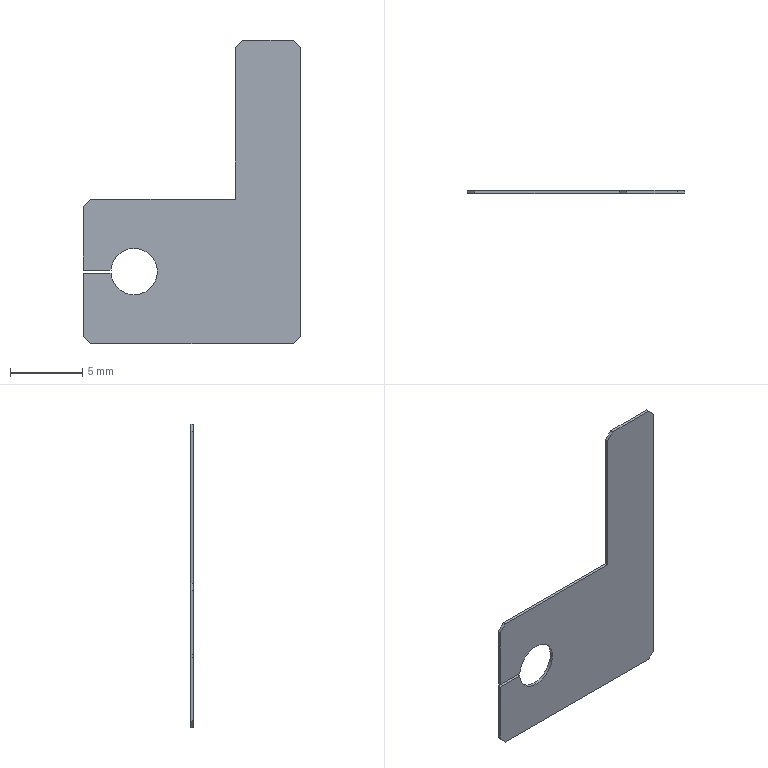Part | SolidWorks | features ICE 3, Chamfer 1, FlatPattern 1, SMBaseFlange 1, SheetMetal 1 | 1 solid | 19 faces | box 15 x 0.2 x 21 mm | volume 38.09 mm3 | plane 16 | cylinder 3 | commonest cylinder face diameters 3.2 x3
STEP:
#1=CARTESIAN_POINT('',(-5.597,0.,5.1));
#2=VERTEX_POINT('',#1);
#3=CARTESIAN_POINT('',(-4.,0.,6.6));
#4=VERTEX_POINT('',#3);
#5=CARTESIAN_POINT('',(-4.,0.,5.));
#6=DIRECTION('',(0.,1.,0.));
#7=DIRECTION('',(0.,0.,1.));
#8=AXIS2_PLACEMENT_3D('',#5,#6,#7);
#9=CIRCLE('',#8,1.6);
#10=EDGE_CURVE('',#2,#4,#9,.T.);
#11=ORIENTED_EDGE('',*,*,#10,.T.);
#12=CARTESIAN_POINT('',(-4.,-0.2,6.6));
#13=VERTEX_POINT('',#12);
#14=CARTESIAN_POINT('',(-4.,9.8,6.6));
#15=DIRECTION('',(0.,-1.,0.));
#16=VECTOR('',#15,1000.);
#17=LINE('',#14,#16);
#18=EDGE_CURVE('',#4,#13,#17,.T.);
#19=ORIENTED_EDGE('',*,*,#18,.T.);
#20=CARTESIAN_POINT('',(-5.597,-0.2,5.1));
#21=VERTEX_POINT('',#20);
#22=CARTESIAN_POINT('',(-4.,-0.2,5.));
#23=DIRECTION('',(0.,-1.,0.));
#24=DIRECTION('',(0.,0.,-1.));
#25=AXIS2_PLACEMENT_3D('',#22,#23,#24);
#26=CIRCLE('',#25,1.6);
#27=EDGE_CURVE('',#13,#21,#26,.T.);
#28=ORIENTED_EDGE('',*,*,#27,.T.);
#29=CARTESIAN_POINT('',(-5.597,0.,5.1));
#30=DIRECTION('',(0.,-1.,0.));
#31=VECTOR('',#30,1000.);
#32=LINE('',#29,#31);
#33=EDGE_CURVE('',#2,#21,#32,.T.);
#34=ORIENTED_EDGE('',*,*,#33,.F.);
#35=EDGE_LOOP('',(#11,#19,#28,#34));
#36=FACE_OUTER_BOUND('',#35,.T.);
#37=CARTESIAN_POINT('',(-4.,9.8,5.));
#38=DIRECTION('',(0.,-1.,0.));
#39=DIRECTION('',(0.,0.,-1.));
#40=AXIS2_PLACEMENT_3D('',#37,#38,#39);
#41=CYLINDRICAL_SURFACE('',#40,1.6);
#42=ADVANCED_FACE('',(#36),#41,.F.);
#43=ORIENTED_EDGE('',*,*,#18,.F.);
#44=CARTESIAN_POINT('',(-4.,0.,3.4));
#45=VERTEX_POINT('',#44);
#46=CARTESIAN_POINT('',(-4.,0.,5.));
#47=DIRECTION('',(0.,1.,0.));
#48=DIRECTION('',(0.,0.,1.));
#49=AXIS2_PLACEMENT_3D('',#46,#47,#48);
#50=CIRCLE('',#49,1.6);
#51=EDGE_CURVE('',#4,#45,#50,.T.);
#52=ORIENTED_EDGE('',*,*,#51,.T.);
#53=CARTESIAN_POINT('',(-4.,-0.2,3.4));
#54=VERTEX_POINT('',#53);
#55=CARTESIAN_POINT('',(-4.,9.8,3.4));
#56=DIRECTION('',(0.,-1.,0.));
#57=VECTOR('',#56,1000.);
#58=LINE('',#55,#57);
#59=EDGE_CURVE('',#45,#54,#58,.T.);
#60=ORIENTED_EDGE('',*,*,#59,.T.);
#61=CARTESIAN_POINT('',(-4.,-0.2,5.));
#62=DIRECTION('',(0.,-1.,0.));
#63=DIRECTION('',(0.,0.,-1.));
#64=AXIS2_PLACEMENT_3D('',#61,#62,#63);
#65=CIRCLE('',#64,1.6);
#66=EDGE_CURVE('',#54,#13,#65,.T.);
#67=ORIENTED_EDGE('',*,*,#66,.T.);
#68=EDGE_LOOP('',(#43,#52,#60,#67));
#69=FACE_OUTER_BOUND('',#68,.T.);
#70=CARTESIAN_POINT('',(-4.,9.8,5.));
#71=DIRECTION('',(0.,-1.,0.));
#72=DIRECTION('',(0.,0.,-1.));
#73=AXIS2_PLACEMENT_3D('',#70,#71,#72);
#74=CYLINDRICAL_SURFACE('',#73,1.6);
#75=ADVANCED_FACE('',(#69),#74,.F.);
#76=CARTESIAN_POINT('',(-7.,-0.2,10.));
#77=VERTEX_POINT('',#76);
#78=CARTESIAN_POINT('',(3.,-0.2,10.));
#79=VERTEX_POINT('',#78);
#80=CARTESIAN_POINT('',(-7.5,-0.2,10.));
#81=DIRECTION('',(1.,0.,0.));
#82=VECTOR('',#81,1000.);
#83=LINE('',#80,#82);
#84=EDGE_CURVE('',#77,#79,#83,.T.);
#85=ORIENTED_EDGE('',*,*,#84,.F.);
#86=CARTESIAN_POINT('',(-7.5,-0.2,9.5));
#87=VERTEX_POINT('',#86);
#88=CARTESIAN_POINT('',(-7.,-0.2,10.));
#89=DIRECTION('',(-0.7071,0.,-0.7071));
#90=VECTOR('',#89,1000.);
#91=LINE('',#88,#90);
#92=EDGE_CURVE('',#77,#87,#91,.T.);
#93=ORIENTED_EDGE('',*,*,#92,.T.);
#94=CARTESIAN_POINT('',(-7.5,-0.2,5.1));
#95=VERTEX_POINT('',#94);
#96=CARTESIAN_POINT('',(-7.5,-0.2,21.));
#97=DIRECTION('',(0.,0.,-1.));
#98=VECTOR('',#97,1000.);
#99=LINE('',#96,#98);
#100=EDGE_CURVE('',#87,#95,#99,.T.);
#101=ORIENTED_EDGE('',*,*,#100,.T.);
#102=CARTESIAN_POINT('',(-7.5,-0.2,5.1));
#103=DIRECTION('',(1.,0.,0.));
#104=VECTOR('',#103,1000.);
#105=LINE('',#102,#104);
#106=EDGE_CURVE('',#95,#21,#105,.T.);
#107=ORIENTED_EDGE('',*,*,#106,.T.);
#108=ORIENTED_EDGE('',*,*,#27,.F.);
#109=ORIENTED_EDGE('',*,*,#66,.F.);
#110=CARTESIAN_POINT('',(-5.597,-0.2,4.9));
#111=VERTEX_POINT('',#110);
#112=CARTESIAN_POINT('',(-4.,-0.2,5.));
#113=DIRECTION('',(0.,-1.,0.));
#114=DIRECTION('',(0.,0.,-1.));
#115=AXIS2_PLACEMENT_3D('',#112,#113,#114);
#116=CIRCLE('',#115,1.6);
#117=EDGE_CURVE('',#111,#54,#116,.T.);
#118=ORIENTED_EDGE('',*,*,#117,.F.);
#119=CARTESIAN_POINT('',(-7.5,-0.2,4.9));
#120=VERTEX_POINT('',#119);
#121=CARTESIAN_POINT('',(-7.5,-0.2,4.9));
#122=DIRECTION('',(-1.,0.,0.));
#123=VECTOR('',#122,1000.);
#124=LINE('',#121,#123);
#125=EDGE_CURVE('',#111,#120,#124,.T.);
#126=ORIENTED_EDGE('',*,*,#125,.T.);
#127=CARTESIAN_POINT('',(-7.5,-0.2,0.5));
#128=VERTEX_POINT('',#127);
#129=CARTESIAN_POINT('',(-7.5,-0.2,21.));
#130=DIRECTION('',(0.,0.,-1.));
#131=VECTOR('',#130,1000.);
#132=LINE('',#129,#131);
#133=EDGE_CURVE('',#120,#128,#132,.T.);
#134=ORIENTED_EDGE('',*,*,#133,.T.);
#135=CARTESIAN_POINT('',(-7.,-0.2,0.));
#136=VERTEX_POINT('',#135);
#137=CARTESIAN_POINT('',(-7.,-0.2,0.));
#138=DIRECTION('',(0.7071,0.,-0.7071));
#139=VECTOR('',#138,1000.);
#140=LINE('',#137,#139);
#141=EDGE_CURVE('',#128,#136,#140,.T.);
#142=ORIENTED_EDGE('',*,*,#141,.T.);
#143=CARTESIAN_POINT('',(7.,-0.2,0.));
#144=VERTEX_POINT('',#143);
#145=CARTESIAN_POINT('',(-7.5,-0.2,0.));
#146=DIRECTION('',(1.,0.,0.));
#147=VECTOR('',#146,1000.);
#148=LINE('',#145,#147);
#149=EDGE_CURVE('',#136,#144,#148,.T.);
#150=ORIENTED_EDGE('',*,*,#149,.T.);
#151=CARTESIAN_POINT('',(7.5,-0.2,0.5));
#152=VERTEX_POINT('',#151);
#153=CARTESIAN_POINT('',(7.,-0.2,0.));
#154=DIRECTION('',(0.7071,0.,0.7071));
#155=VECTOR('',#154,1000.);
#156=LINE('',#153,#155);
#157=EDGE_CURVE('',#144,#152,#156,.T.);
#158=ORIENTED_EDGE('',*,*,#157,.T.);
#159=CARTESIAN_POINT('',(7.5,-0.2,20.5));
#160=VERTEX_POINT('',#159);
#161=CARTESIAN_POINT('',(7.5,-0.2,21.));
#162=DIRECTION('',(0.,0.,-1.));
#163=VECTOR('',#162,1000.);
#164=LINE('',#161,#163);
#165=EDGE_CURVE('',#160,#152,#164,.T.);
#166=ORIENTED_EDGE('',*,*,#165,.F.);
#167=CARTESIAN_POINT('',(7.,-0.2,21.));
#168=VERTEX_POINT('',#167);
#169=CARTESIAN_POINT('',(7.5,-0.2,20.5));
#170=DIRECTION('',(-0.7071,0.,0.7071));
#171=VECTOR('',#170,1000.);
#172=LINE('',#169,#171);
#173=EDGE_CURVE('',#160,#168,#172,.T.);
#174=ORIENTED_EDGE('',*,*,#173,.T.);
#175=CARTESIAN_POINT('',(3.5,-0.2,21.));
#176=VERTEX_POINT('',#175);
#177=CARTESIAN_POINT('',(-7.5,-0.2,21.));
#178=DIRECTION('',(1.,0.,0.));
#179=VECTOR('',#178,1000.);
#180=LINE('',#177,#179);
#181=EDGE_CURVE('',#176,#168,#180,.T.);
#182=ORIENTED_EDGE('',*,*,#181,.F.);
#183=CARTESIAN_POINT('',(3.,-0.2,20.5));
#184=VERTEX_POINT('',#183);
#185=CARTESIAN_POINT('',(3.5,-0.2,21.));
#186=DIRECTION('',(-0.7071,0.,-0.7071));
#187=VECTOR('',#186,1000.);
#188=LINE('',#185,#187);
#189=EDGE_CURVE('',#176,#184,#188,.T.);
#190=ORIENTED_EDGE('',*,*,#189,.T.);
#191=CARTESIAN_POINT('',(3.,-0.2,21.));
#192=DIRECTION('',(0.,0.,1.));
#193=VECTOR('',#192,1000.);
#194=LINE('',#191,#193);
#195=EDGE_CURVE('',#79,#184,#194,.T.);
#196=ORIENTED_EDGE('',*,*,#195,.F.);
#197=EDGE_LOOP('',(#85,#93,#101,#107,#108,#109,#118,#126,#134,#142,#150,#158,#166,#174,#182,#190,#196));
#198=FACE_OUTER_BOUND('',#197,.T.);
#199=CARTESIAN_POINT('',(-7.5,-0.2,21.));
#200=DIRECTION('',(0.,1.,0.));
#201=DIRECTION('',(0.,0.,1.));
#202=AXIS2_PLACEMENT_3D('',#199,#200,#201);
#203=PLANE('',#202);
#204=ADVANCED_FACE('',(#198),#203,.F.);
#205=CARTESIAN_POINT('',(-7.5,0.,9.5));
#206=VERTEX_POINT('',#205);
#207=CARTESIAN_POINT('',(-7.5,0.,5.1));
#208=VERTEX_POINT('',#207);
#209=CARTESIAN_POINT('',(-7.5,0.,21.));
#210=DIRECTION('',(0.,0.,-1.));
#211=VECTOR('',#210,1000.);
#212=LINE('',#209,#211);
#213=EDGE_CURVE('',#206,#208,#212,.T.);
#214=ORIENTED_EDGE('',*,*,#213,.F.);
#215=CARTESIAN_POINT('',(-7.,0.,10.));
#216=VERTEX_POINT('',#215);
#217=CARTESIAN_POINT('',(-1.75,0.,15.25));
#218=DIRECTION('',(0.7071,0.,0.7071));
#219=VECTOR('',#218,1000.);
#220=LINE('',#217,#219);
#221=EDGE_CURVE('',#206,#216,#220,.T.);
#222=ORIENTED_EDGE('',*,*,#221,.T.);
#223=CARTESIAN_POINT('',(3.,0.,10.));
#224=VERTEX_POINT('',#223);
#225=CARTESIAN_POINT('',(-7.5,0.,10.));
#226=DIRECTION('',(-1.,0.,0.));
#227=VECTOR('',#226,1000.);
#228=LINE('',#225,#227);
#229=EDGE_CURVE('',#224,#216,#228,.T.);
#230=ORIENTED_EDGE('',*,*,#229,.F.);
#231=CARTESIAN_POINT('',(3.,0.,20.5));
#232=VERTEX_POINT('',#231);
#233=CARTESIAN_POINT('',(3.,0.,21.));
#234=DIRECTION('',(0.,0.,-1.));
#235=VECTOR('',#234,1000.);
#236=LINE('',#233,#235);
#237=EDGE_CURVE('',#232,#224,#236,.T.);
#238=ORIENTED_EDGE('',*,*,#237,.F.);
#239=CARTESIAN_POINT('',(3.5,0.,21.));
#240=VERTEX_POINT('',#239);
#241=CARTESIAN_POINT('',(-2.,0.,15.5));
#242=DIRECTION('',(0.7071,0.,0.7071));
#243=VECTOR('',#242,1000.);
#244=LINE('',#241,#243);
#245=EDGE_CURVE('',#232,#240,#244,.T.);
#246=ORIENTED_EDGE('',*,*,#245,.T.);
#247=CARTESIAN_POINT('',(7.,0.,21.));
#248=VERTEX_POINT('',#247);
#249=CARTESIAN_POINT('',(-7.5,0.,21.));
#250=DIRECTION('',(1.,0.,0.));
#251=VECTOR('',#250,1000.);
#252=LINE('',#249,#251);
#253=EDGE_CURVE('',#240,#248,#252,.T.);
#254=ORIENTED_EDGE('',*,*,#253,.T.);
#255=CARTESIAN_POINT('',(7.5,0.,20.5));
#256=VERTEX_POINT('',#255);
#257=CARTESIAN_POINT('',(-0.25,0.,28.25));
#258=DIRECTION('',(0.7071,0.,-0.7071));
#259=VECTOR('',#258,1000.);
#260=LINE('',#257,#259);
#261=EDGE_CURVE('',#248,#256,#260,.T.);
#262=ORIENTED_EDGE('',*,*,#261,.T.);
#263=CARTESIAN_POINT('',(7.5,0.,0.5));
#264=VERTEX_POINT('',#263);
#265=CARTESIAN_POINT('',(7.5,0.,21.));
#266=DIRECTION('',(0.,0.,-1.));
#267=VECTOR('',#266,1000.);
#268=LINE('',#265,#267);
#269=EDGE_CURVE('',#256,#264,#268,.T.);
#270=ORIENTED_EDGE('',*,*,#269,.T.);
#271=CARTESIAN_POINT('',(7.,0.,0.));
#272=VERTEX_POINT('',#271);
#273=CARTESIAN_POINT('',(10.25,0.,3.25));
#274=DIRECTION('',(-0.7071,0.,-0.7071));
#275=VECTOR('',#274,1000.);
#276=LINE('',#273,#275);
#277=EDGE_CURVE('',#264,#272,#276,.T.);
#278=ORIENTED_EDGE('',*,*,#277,.T.);
#279=CARTESIAN_POINT('',(-7.,0.,0.));
#280=VERTEX_POINT('',#279);
#281=CARTESIAN_POINT('',(-7.5,0.,0.));
#282=DIRECTION('',(1.,0.,0.));
#283=VECTOR('',#282,1000.);
#284=LINE('',#281,#283);
#285=EDGE_CURVE('',#280,#272,#284,.T.);
#286=ORIENTED_EDGE('',*,*,#285,.F.);
#287=CARTESIAN_POINT('',(-7.5,0.,0.5));
#288=VERTEX_POINT('',#287);
#289=CARTESIAN_POINT('',(-17.75,0.,10.75));
#290=DIRECTION('',(-0.7071,0.,0.7071));
#291=VECTOR('',#290,1000.);
#292=LINE('',#289,#291);
#293=EDGE_CURVE('',#280,#288,#292,.T.);
#294=ORIENTED_EDGE('',*,*,#293,.T.);
#295=CARTESIAN_POINT('',(-7.5,0.,4.9));
#296=VERTEX_POINT('',#295);
#297=CARTESIAN_POINT('',(-7.5,0.,21.));
#298=DIRECTION('',(0.,0.,-1.));
#299=VECTOR('',#298,1000.);
#300=LINE('',#297,#299);
#301=EDGE_CURVE('',#296,#288,#300,.T.);
#302=ORIENTED_EDGE('',*,*,#301,.F.);
#303=CARTESIAN_POINT('',(-5.597,0.,4.9));
#304=VERTEX_POINT('',#303);
#305=CARTESIAN_POINT('',(-7.5,0.,4.9));
#306=DIRECTION('',(-1.,0.,0.));
#307=VECTOR('',#306,1000.);
#308=LINE('',#305,#307);
#309=EDGE_CURVE('',#304,#296,#308,.T.);
#310=ORIENTED_EDGE('',*,*,#309,.F.);
#311=CARTESIAN_POINT('',(-4.,0.,5.));
#312=DIRECTION('',(0.,1.,0.));
#313=DIRECTION('',(0.,0.,1.));
#314=AXIS2_PLACEMENT_3D('',#311,#312,#313);
#315=CIRCLE('',#314,1.6);
#316=EDGE_CURVE('',#45,#304,#315,.T.);
#317=ORIENTED_EDGE('',*,*,#316,.F.);
#318=ORIENTED_EDGE('',*,*,#51,.F.);
#319=ORIENTED_EDGE('',*,*,#10,.F.);
#320=CARTESIAN_POINT('',(-7.5,0.,5.1));
#321=DIRECTION('',(1.,0.,0.));
#322=VECTOR('',#321,1000.);
#323=LINE('',#320,#322);
#324=EDGE_CURVE('',#208,#2,#323,.T.);
#325=ORIENTED_EDGE('',*,*,#324,.F.);
#326=EDGE_LOOP('',(#214,#222,#230,#238,#246,#254,#262,#270,#278,#286,#294,#302,#310,#317,#318,#319,#325));
#327=FACE_OUTER_BOUND('',#326,.T.);
#328=CARTESIAN_POINT('',(-7.5,0.,21.));
#329=DIRECTION('',(0.,1.,0.));
#330=DIRECTION('',(0.,0.,1.));
#331=AXIS2_PLACEMENT_3D('',#328,#329,#330);
#332=PLANE('',#331);
#333=ADVANCED_FACE('',(#327),#332,.T.);
#334=ORIENTED_EDGE('',*,*,#301,.T.);
#335=CARTESIAN_POINT('',(-7.5,-0.2,0.5));
#336=DIRECTION('',(0.,-1.,0.));
#337=VECTOR('',#336,1000.);
#338=LINE('',#335,#337);
#339=EDGE_CURVE('',#288,#128,#338,.T.);
#340=ORIENTED_EDGE('',*,*,#339,.T.);
#341=ORIENTED_EDGE('',*,*,#133,.F.);
#342=CARTESIAN_POINT('',(-7.5,0.,4.9));
#343=DIRECTION('',(0.,-1.,0.));
#344=VECTOR('',#343,1000.);
#345=LINE('',#342,#344);
#346=EDGE_CURVE('',#296,#120,#345,.T.);
#347=ORIENTED_EDGE('',*,*,#346,.F.);
#348=EDGE_LOOP('',(#334,#340,#341,#347));
#349=FACE_OUTER_BOUND('',#348,.T.);
#350=CARTESIAN_POINT('',(-7.5,-0.2,21.));
#351=DIRECTION('',(-1.,0.,0.));
#352=DIRECTION('',(0.,0.,1.));
#353=AXIS2_PLACEMENT_3D('',#350,#351,#352);
#354=PLANE('',#353);
#355=ADVANCED_FACE('',(#349),#354,.T.);
#356=ORIENTED_EDGE('',*,*,#100,.F.);
#357=CARTESIAN_POINT('',(-7.5,0.,9.5));
#358=DIRECTION('',(0.,1.,0.));
#359=VECTOR('',#358,1000.);
#360=LINE('',#357,#359);
#361=EDGE_CURVE('',#87,#206,#360,.T.);
#362=ORIENTED_EDGE('',*,*,#361,.T.);
#363=ORIENTED_EDGE('',*,*,#213,.T.);
#364=CARTESIAN_POINT('',(-7.5,0.,5.1));
#365=DIRECTION('',(0.,-1.,0.));
#366=VECTOR('',#365,1000.);
#367=LINE('',#364,#366);
#368=EDGE_CURVE('',#208,#95,#367,.T.);
#369=ORIENTED_EDGE('',*,*,#368,.T.);
#370=EDGE_LOOP('',(#356,#362,#363,#369));
#371=FACE_OUTER_BOUND('',#370,.T.);
#372=CARTESIAN_POINT('',(-7.5,-0.2,21.));
#373=DIRECTION('',(-1.,0.,0.));
#374=DIRECTION('',(0.,0.,1.));
#375=AXIS2_PLACEMENT_3D('',#372,#373,#374);
#376=PLANE('',#375);
#377=ADVANCED_FACE('',(#371),#376,.T.);
#378=ORIENTED_EDGE('',*,*,#59,.F.);
#379=ORIENTED_EDGE('',*,*,#316,.T.);
#380=CARTESIAN_POINT('',(-5.597,0.,4.9));
#381=DIRECTION('',(0.,-1.,0.));
#382=VECTOR('',#381,1000.);
#383=LINE('',#380,#382);
#384=EDGE_CURVE('',#304,#111,#383,.T.);
#385=ORIENTED_EDGE('',*,*,#384,.T.);
#386=ORIENTED_EDGE('',*,*,#117,.T.);
#387=EDGE_LOOP('',(#378,#379,#385,#386));
#388=FACE_OUTER_BOUND('',#387,.T.);
#389=CARTESIAN_POINT('',(-4.,9.8,5.));
#390=DIRECTION('',(0.,-1.,0.));
#391=DIRECTION('',(0.,0.,-1.));
#392=AXIS2_PLACEMENT_3D('',#389,#390,#391);
#393=CYLINDRICAL_SURFACE('',#392,1.6);
#394=ADVANCED_FACE('',(#388),#393,.F.);
#395=ORIENTED_EDGE('',*,*,#165,.T.);
#396=CARTESIAN_POINT('',(7.5,0.,0.5));
#397=DIRECTION('',(0.,1.,0.));
#398=VECTOR('',#397,1000.);
#399=LINE('',#396,#398);
#400=EDGE_CURVE('',#152,#264,#399,.T.);
#401=ORIENTED_EDGE('',*,*,#400,.T.);
#402=ORIENTED_EDGE('',*,*,#269,.F.);
#403=CARTESIAN_POINT('',(7.5,-0.2,20.5));
#404=DIRECTION('',(0.,-1.,0.));
#405=VECTOR('',#404,1000.);
#406=LINE('',#403,#405);
#407=EDGE_CURVE('',#256,#160,#406,.T.);
#408=ORIENTED_EDGE('',*,*,#407,.T.);
#409=EDGE_LOOP('',(#395,#401,#402,#408));
#410=FACE_OUTER_BOUND('',#409,.T.);
#411=CARTESIAN_POINT('',(7.5,0.,21.));
#412=DIRECTION('',(1.,0.,0.));
#413=DIRECTION('',(0.,0.,-1.));
#414=AXIS2_PLACEMENT_3D('',#411,#412,#413);
#415=PLANE('',#414);
#416=ADVANCED_FACE('',(#410),#415,.T.);
#417=ORIENTED_EDGE('',*,*,#253,.F.);
#418=CARTESIAN_POINT('',(3.5,0.,21.));
#419=DIRECTION('',(0.,-1.,0.));
#420=VECTOR('',#419,1000.);
#421=LINE('',#418,#420);
#422=EDGE_CURVE('',#240,#176,#421,.T.);
#423=ORIENTED_EDGE('',*,*,#422,.T.);
#424=ORIENTED_EDGE('',*,*,#181,.T.);
#425=CARTESIAN_POINT('',(7.,0.,21.));
#426=DIRECTION('',(0.,1.,0.));
#427=VECTOR('',#426,1000.);
#428=LINE('',#425,#427);
#429=EDGE_CURVE('',#168,#248,#428,.T.);
#430=ORIENTED_EDGE('',*,*,#429,.T.);
#431=EDGE_LOOP('',(#417,#423,#424,#430));
#432=FACE_OUTER_BOUND('',#431,.T.);
#433=CARTESIAN_POINT('',(0.,0.,21.));
#434=DIRECTION('',(0.,0.,-1.));
#435=DIRECTION('',(-1.,0.,0.));
#436=AXIS2_PLACEMENT_3D('',#433,#434,#435);
#437=PLANE('',#436);
#438=ADVANCED_FACE('',(#432),#437,.F.);
#439=ORIENTED_EDGE('',*,*,#149,.F.);
#440=CARTESIAN_POINT('',(-7.,0.,0.));
#441=DIRECTION('',(0.,1.,0.));
#442=VECTOR('',#441,1000.);
#443=LINE('',#440,#442);
#444=EDGE_CURVE('',#136,#280,#443,.T.);
#445=ORIENTED_EDGE('',*,*,#444,.T.);
#446=ORIENTED_EDGE('',*,*,#285,.T.);
#447=CARTESIAN_POINT('',(7.,0.,0.));
#448=DIRECTION('',(0.,-1.,0.));
#449=VECTOR('',#448,1000.);
#450=LINE('',#447,#449);
#451=EDGE_CURVE('',#272,#144,#450,.T.);
#452=ORIENTED_EDGE('',*,*,#451,.T.);
#453=EDGE_LOOP('',(#439,#445,#446,#452));
#454=FACE_OUTER_BOUND('',#453,.T.);
#455=CARTESIAN_POINT('',(0.,0.,0.));
#456=DIRECTION('',(0.,0.,-1.));
#457=DIRECTION('',(-1.,0.,0.));
#458=AXIS2_PLACEMENT_3D('',#455,#456,#457);
#459=PLANE('',#458);
#460=ADVANCED_FACE('',(#454),#459,.T.);
#461=ORIENTED_EDGE('',*,*,#195,.T.);
#462=CARTESIAN_POINT('',(3.,9.8,20.5));
#463=DIRECTION('',(0.,1.,0.));
#464=VECTOR('',#463,1000.);
#465=LINE('',#462,#464);
#466=EDGE_CURVE('',#184,#232,#465,.T.);
#467=ORIENTED_EDGE('',*,*,#466,.T.);
#468=ORIENTED_EDGE('',*,*,#237,.T.);
#469=CARTESIAN_POINT('',(3.,9.8,10.));
#470=DIRECTION('',(0.,-1.,0.));
#471=VECTOR('',#470,1000.);
#472=LINE('',#469,#471);
#473=EDGE_CURVE('',#224,#79,#472,.T.);
#474=ORIENTED_EDGE('',*,*,#473,.T.);
#475=EDGE_LOOP('',(#461,#467,#468,#474));
#476=FACE_OUTER_BOUND('',#475,.T.);
#477=CARTESIAN_POINT('',(3.,9.8,21.));
#478=DIRECTION('',(1.,0.,0.));
#479=DIRECTION('',(0.,0.,-1.));
#480=AXIS2_PLACEMENT_3D('',#477,#478,#479);
#481=PLANE('',#480);
#482=ADVANCED_FACE('',(#476),#481,.F.);
#483=ORIENTED_EDGE('',*,*,#229,.T.);
#484=CARTESIAN_POINT('',(-7.,-0.2,10.));
#485=DIRECTION('',(0.,-1.,0.));
#486=VECTOR('',#485,1000.);
#487=LINE('',#484,#486);
#488=EDGE_CURVE('',#216,#77,#487,.T.);
#489=ORIENTED_EDGE('',*,*,#488,.T.);
#490=ORIENTED_EDGE('',*,*,#84,.T.);
#491=ORIENTED_EDGE('',*,*,#473,.F.);
#492=EDGE_LOOP('',(#483,#489,#490,#491));
#493=FACE_OUTER_BOUND('',#492,.T.);
#494=CARTESIAN_POINT('',(-7.5,9.8,10.));
#495=DIRECTION('',(0.,0.,-1.));
#496=DIRECTION('',(-1.,0.,0.));
#497=AXIS2_PLACEMENT_3D('',#494,#495,#496);
#498=PLANE('',#497);
#499=ADVANCED_FACE('',(#493),#498,.F.);
#500=ORIENTED_EDGE('',*,*,#324,.T.);
#501=ORIENTED_EDGE('',*,*,#33,.T.);
#502=ORIENTED_EDGE('',*,*,#106,.F.);
#503=ORIENTED_EDGE('',*,*,#368,.F.);
#504=EDGE_LOOP('',(#500,#501,#502,#503));
#505=FACE_OUTER_BOUND('',#504,.T.);
#506=CARTESIAN_POINT('',(-7.5,0.,5.1));
#507=DIRECTION('',(0.,0.,1.));
#508=DIRECTION('',(1.,0.,0.));
#509=AXIS2_PLACEMENT_3D('',#506,#507,#508);
#510=PLANE('',#509);
#511=ADVANCED_FACE('',(#505),#510,.F.);
#512=ORIENTED_EDGE('',*,*,#384,.F.);
#513=ORIENTED_EDGE('',*,*,#309,.T.);
#514=ORIENTED_EDGE('',*,*,#346,.T.);
#515=ORIENTED_EDGE('',*,*,#125,.F.);
#516=EDGE_LOOP('',(#512,#513,#514,#515));
#517=FACE_OUTER_BOUND('',#516,.T.);
#518=CARTESIAN_POINT('',(-7.5,0.,4.9));
#519=DIRECTION('',(0.,0.,-1.));
#520=DIRECTION('',(-1.,0.,0.));
#521=AXIS2_PLACEMENT_3D('',#518,#519,#520);
#522=PLANE('',#521);
#523=ADVANCED_FACE('',(#517),#522,.F.);
#524=ORIENTED_EDGE('',*,*,#221,.F.);
#525=ORIENTED_EDGE('',*,*,#361,.F.);
#526=ORIENTED_EDGE('',*,*,#92,.F.);
#527=ORIENTED_EDGE('',*,*,#488,.F.);
#528=EDGE_LOOP('',(#524,#525,#526,#527));
#529=FACE_OUTER_BOUND('',#528,.T.);
#530=CARTESIAN_POINT('',(-7.,9.8,10.));
#531=DIRECTION('',(-0.7071,0.,0.7071));
#532=DIRECTION('',(0.,1.,0.));
#533=AXIS2_PLACEMENT_3D('',#530,#531,#532);
#534=PLANE('',#533);
#535=ADVANCED_FACE('',(#529),#534,.T.);
#536=ORIENTED_EDGE('',*,*,#141,.F.);
#537=ORIENTED_EDGE('',*,*,#339,.F.);
#538=ORIENTED_EDGE('',*,*,#293,.F.);
#539=ORIENTED_EDGE('',*,*,#444,.F.);
#540=EDGE_LOOP('',(#536,#537,#538,#539));
#541=FACE_OUTER_BOUND('',#540,.T.);
#542=CARTESIAN_POINT('',(-7.,0.,0.));
#543=DIRECTION('',(0.7071,0.,0.7071));
#544=DIRECTION('',(0.,1.,0.));
#545=AXIS2_PLACEMENT_3D('',#542,#543,#544);
#546=PLANE('',#545);
#547=ADVANCED_FACE('',(#541),#546,.F.);
#548=ORIENTED_EDGE('',*,*,#277,.F.);
#549=ORIENTED_EDGE('',*,*,#400,.F.);
#550=ORIENTED_EDGE('',*,*,#157,.F.);
#551=ORIENTED_EDGE('',*,*,#451,.F.);
#552=EDGE_LOOP('',(#548,#549,#550,#551));
#553=FACE_OUTER_BOUND('',#552,.T.);
#554=CARTESIAN_POINT('',(7.,0.,0.));
#555=DIRECTION('',(-0.7071,0.,0.7071));
#556=DIRECTION('',(0.,-1.,0.));
#557=AXIS2_PLACEMENT_3D('',#554,#555,#556);
#558=PLANE('',#557);
#559=ADVANCED_FACE('',(#553),#558,.F.);
#560=ORIENTED_EDGE('',*,*,#245,.F.);
#561=ORIENTED_EDGE('',*,*,#466,.F.);
#562=ORIENTED_EDGE('',*,*,#189,.F.);
#563=ORIENTED_EDGE('',*,*,#422,.F.);
#564=EDGE_LOOP('',(#560,#561,#562,#563));
#565=FACE_OUTER_BOUND('',#564,.T.);
#566=CARTESIAN_POINT('',(3.5,0.,21.));
#567=DIRECTION('',(0.7071,0.,-0.7071));
#568=DIRECTION('',(0.,-1.,0.));
#569=AXIS2_PLACEMENT_3D('',#566,#567,#568);
#570=PLANE('',#569);
#571=ADVANCED_FACE('',(#565),#570,.F.);
#572=ORIENTED_EDGE('',*,*,#261,.F.);
#573=ORIENTED_EDGE('',*,*,#429,.F.);
#574=ORIENTED_EDGE('',*,*,#173,.F.);
#575=ORIENTED_EDGE('',*,*,#407,.F.);
#576=EDGE_LOOP('',(#572,#573,#574,#575));
#577=FACE_OUTER_BOUND('',#576,.T.);
#578=CARTESIAN_POINT('',(7.5,0.,20.5));
#579=DIRECTION('',(0.7071,0.,0.7071));
#580=DIRECTION('',(0.,1.,0.));
#581=AXIS2_PLACEMENT_3D('',#578,#579,#580);
#582=PLANE('',#581);
#583=ADVANCED_FACE('',(#577),#582,.T.);
#584=CLOSED_SHELL('',(#42,#75,#204,#333,#355,#377,#394,#416,#438,#460,#482,#499,#511,#523,#535,#547,#559,#571,#583));
#585=MANIFOLD_SOLID_BREP('',#584);
#586=CARTESIAN_POINT('',(0.,0.,0.));
#587=DIRECTION('',(0.,0.,1.));
#588=DIRECTION('',(1.,0.,0.));
#589=AXIS2_PLACEMENT_3D('',#586,#587,#588);
#590=(LENGTH_UNIT()NAMED_UNIT(*)SI_UNIT(.MILLI.,.METRE.));
#591=UNCERTAINTY_MEASURE_WITH_UNIT(LENGTH_MEASURE(0.00001),#590,'','');
#592=(NAMED_UNIT(*)PLANE_ANGLE_UNIT()SI_UNIT($,.RADIAN.));
#593=(NAMED_UNIT(*)SI_UNIT($,.STERADIAN.)SOLID_ANGLE_UNIT());
#594=(GEOMETRIC_REPRESENTATION_CONTEXT(3)GLOBAL_UNCERTAINTY_ASSIGNED_CONTEXT((#591))GLOBAL_UNIT_ASSIGNED_CONTEXT((#590,#592,#593))REPRESENTATION_CONTEXT('',''));
#595=ADVANCED_BREP_SHAPE_REPRESENTATION('',(#585,#589),#594);